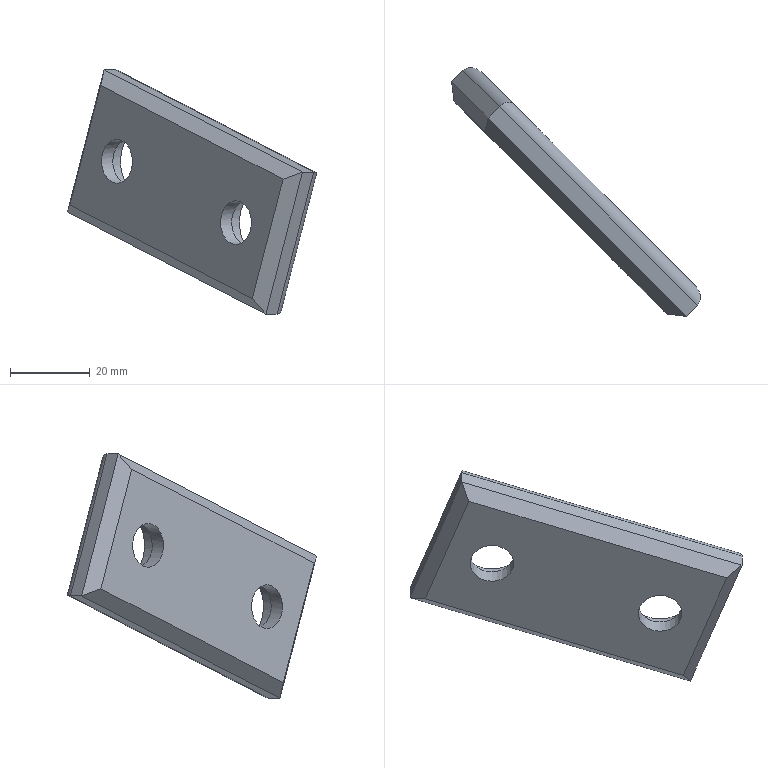Part | NX | features solid 2 | 1 solid | 20 faces | box 62.583 x 62.583 x 61.36 mm | volume 23446 mm3 | plane 12 | cylinder 8 | commonest cylinder face diameters 6 x4 11 x2 17.5 x2
STEP:
#1=CARTESIAN_POINT('',(-428.02,835.996,-99.293));
#2=VERTEX_POINT('',#1);
#3=CARTESIAN_POINT('',(-425.192,838.824,-99.293));
#4=VERTEX_POINT('',#3);
#5=CARTESIAN_POINT('',(-437.213,826.803,-99.293));
#6=DIRECTION('',(0.7071,0.7071,0.));
#7=VECTOR('',#6,1000.);
#8=LINE('',#5,#7);
#9=EDGE_CURVE('',#2,#4,#8,.T.);
#10=ORIENTED_EDGE('',*,*,#9,.F.);
#11=CARTESIAN_POINT('',(-418.83,826.806,-63.585));
#12=VERTEX_POINT('',#11);
#13=CARTESIAN_POINT('',(-428.02,835.996,-99.293));
#14=DIRECTION('',(0.2418,-0.2418,0.9397));
#15=VECTOR('',#14,1000.);
#16=LINE('',#13,#15);
#17=EDGE_CURVE('',#2,#12,#16,.T.);
#18=ORIENTED_EDGE('',*,*,#17,.T.);
#19=CARTESIAN_POINT('',(-416.002,829.634,-63.585));
#20=VERTEX_POINT('',#19);
#21=CARTESIAN_POINT('',(-428.022,817.613,-63.585));
#22=DIRECTION('',(0.7071,0.7071,0.));
#23=VECTOR('',#22,1000.);
#24=LINE('',#21,#23);
#25=EDGE_CURVE('',#12,#20,#24,.T.);
#26=ORIENTED_EDGE('',*,*,#25,.T.);
#27=CARTESIAN_POINT('',(-418.42,832.053,-72.982));
#28=DIRECTION('',(-0.2418,0.2418,-0.9397));
#29=VECTOR('',#28,1000.);
#30=LINE('',#27,#29);
#31=EDGE_CURVE('',#20,#4,#30,.T.);
#32=ORIENTED_EDGE('',*,*,#31,.T.);
#33=EDGE_LOOP('',(#10,#18,#26,#32));
#34=FACE_BOUND('',#33,.T.);
#35=CARTESIAN_POINT('',(-430.441,820.032,-72.982));
#36=DIRECTION('',(0.6645,-0.6645,-0.342));
#37=DIRECTION('',(0.7071,0.7071,0.));
#38=AXIS2_PLACEMENT_3D('',#35,#36,#37);
#39=PLANE('',#38);
#40=ADVANCED_FACE('',(#34),#39,.F.);
#41=CARTESIAN_POINT('',(-378.185,786.161,-124.945));
#42=VERTEX_POINT('',#41);
#43=CARTESIAN_POINT('',(-375.357,788.989,-124.945));
#44=VERTEX_POINT('',#43);
#45=CARTESIAN_POINT('',(-387.378,776.969,-124.945));
#46=DIRECTION('',(0.7071,0.7071,0.));
#47=VECTOR('',#46,1000.);
#48=LINE('',#45,#47);
#49=EDGE_CURVE('',#42,#44,#48,.T.);
#50=ORIENTED_EDGE('',*,*,#49,.F.);
#51=CARTESIAN_POINT('',(-428.02,835.996,-99.293));
#52=DIRECTION('',(-0.6645,0.6645,0.342));
#53=VECTOR('',#52,1000.);
#54=LINE('',#51,#53);
#55=EDGE_CURVE('',#42,#2,#54,.T.);
#56=ORIENTED_EDGE('',*,*,#55,.T.);
#57=ORIENTED_EDGE('',*,*,#9,.T.);
#58=CARTESIAN_POINT('',(-425.192,838.824,-99.293));
#59=DIRECTION('',(0.6645,-0.6645,-0.342));
#60=VECTOR('',#59,1000.);
#61=LINE('',#58,#60);
#62=EDGE_CURVE('',#4,#44,#61,.T.);
#63=ORIENTED_EDGE('',*,*,#62,.T.);
#64=EDGE_LOOP('',(#50,#56,#57,#63));
#65=FACE_BOUND('',#64,.T.);
#66=CARTESIAN_POINT('',(-437.213,826.803,-99.293));
#67=DIRECTION('',(0.2418,-0.2418,0.9397));
#68=DIRECTION('',(-0.7071,-0.7071,0.));
#69=AXIS2_PLACEMENT_3D('',#66,#67,#68);
#70=PLANE('',#69);
#71=ADVANCED_FACE('',(#65),#70,.F.);
#72=CARTESIAN_POINT('',(-368.995,776.971,-89.236));
#73=VERTEX_POINT('',#72);
#74=CARTESIAN_POINT('',(-366.167,779.799,-89.236));
#75=VERTEX_POINT('',#74);
#76=CARTESIAN_POINT('',(-378.188,767.779,-89.236));
#77=DIRECTION('',(0.7071,0.7071,0.));
#78=VECTOR('',#77,1000.);
#79=LINE('',#76,#78);
#80=EDGE_CURVE('',#73,#75,#79,.T.);
#81=ORIENTED_EDGE('',*,*,#80,.F.);
#82=CARTESIAN_POINT('',(-378.185,786.161,-124.945));
#83=DIRECTION('',(-0.2418,0.2418,-0.9397));
#84=VECTOR('',#83,1000.);
#85=LINE('',#82,#84);
#86=EDGE_CURVE('',#73,#42,#85,.T.);
#87=ORIENTED_EDGE('',*,*,#86,.T.);
#88=ORIENTED_EDGE('',*,*,#49,.T.);
#89=CARTESIAN_POINT('',(-375.357,788.989,-124.945));
#90=DIRECTION('',(0.2418,-0.2418,0.9397));
#91=VECTOR('',#90,1000.);
#92=LINE('',#89,#91);
#93=EDGE_CURVE('',#44,#75,#92,.T.);
#94=ORIENTED_EDGE('',*,*,#93,.T.);
#95=EDGE_LOOP('',(#81,#87,#88,#94));
#96=FACE_BOUND('',#95,.T.);
#97=CARTESIAN_POINT('',(-387.378,776.969,-124.945));
#98=DIRECTION('',(-0.6645,0.6645,0.342));
#99=DIRECTION('',(-0.7071,-0.7071,0.));
#100=AXIS2_PLACEMENT_3D('',#97,#98,#99);
#101=PLANE('',#100);
#102=ADVANCED_FACE('',(#96),#101,.F.);
#103=ORIENTED_EDGE('',*,*,#25,.F.);
#104=CARTESIAN_POINT('',(-418.83,826.806,-63.585));
#105=DIRECTION('',(0.6645,-0.6645,-0.342));
#106=VECTOR('',#105,1000.);
#107=LINE('',#104,#106);
#108=EDGE_CURVE('',#12,#73,#107,.T.);
#109=ORIENTED_EDGE('',*,*,#108,.T.);
#110=ORIENTED_EDGE('',*,*,#80,.T.);
#111=CARTESIAN_POINT('',(-366.167,779.799,-89.236));
#112=DIRECTION('',(-0.6645,0.6645,0.342));
#113=VECTOR('',#112,1000.);
#114=LINE('',#111,#113);
#115=EDGE_CURVE('',#75,#20,#114,.T.);
#116=ORIENTED_EDGE('',*,*,#115,.T.);
#117=EDGE_LOOP('',(#103,#109,#110,#116));
#118=FACE_BOUND('',#117,.T.);
#119=CARTESIAN_POINT('',(-378.188,767.779,-89.236));
#120=DIRECTION('',(-0.2418,0.2418,-0.9397));
#121=DIRECTION('',(0.6645,-0.6645,-0.342));
#122=AXIS2_PLACEMENT_3D('',#119,#120,#121);
#123=PLANE('',#122);
#124=ADVANCED_FACE('',(#118),#123,.F.);
#125=CARTESIAN_POINT('',(-427.423,831.155,-97.5));
#126=VERTEX_POINT('',#125);
#127=CARTESIAN_POINT('',(-381.575,785.308,-121.1));
#128=VERTEX_POINT('',#127);
#129=CARTESIAN_POINT('',(-379.581,783.314,-122.126));
#130=DIRECTION('',(0.6645,-0.6645,-0.342));
#131=VECTOR('',#130,1000.);
#132=LINE('',#129,#131);
#133=EDGE_CURVE('',#126,#128,#132,.T.);
#134=ORIENTED_EDGE('',*,*,#133,.T.);
#135=CARTESIAN_POINT('',(-373.836,777.569,-91.029));
#136=VERTEX_POINT('',#135);
#137=CARTESIAN_POINT('',(-375.529,779.261,-97.607));
#138=DIRECTION('',(0.2418,-0.2418,0.9397));
#139=VECTOR('',#138,1000.);
#140=LINE('',#137,#139);
#141=EDGE_CURVE('',#128,#136,#140,.T.);
#142=ORIENTED_EDGE('',*,*,#141,.T.);
#143=CARTESIAN_POINT('',(-419.684,823.416,-67.43));
#144=VERTEX_POINT('',#143);
#145=CARTESIAN_POINT('',(-421.677,825.41,-66.404));
#146=DIRECTION('',(-0.6645,0.6645,0.342));
#147=VECTOR('',#146,1000.);
#148=LINE('',#145,#147);
#149=EDGE_CURVE('',#136,#144,#148,.T.);
#150=ORIENTED_EDGE('',*,*,#149,.T.);
#151=CARTESIAN_POINT('',(-428.148,831.881,-100.319));
#152=DIRECTION('',(-0.2418,0.2418,-0.9397));
#153=VECTOR('',#152,1000.);
#154=LINE('',#151,#153);
#155=EDGE_CURVE('',#144,#126,#154,.T.);
#156=ORIENTED_EDGE('',*,*,#155,.T.);
#157=EDGE_LOOP('',(#134,#142,#150,#156));
#158=FACE_BOUND('',#157,.T.);
#159=CARTESIAN_POINT('',(-382.024,785.757,-103.841));
#160=VERTEX_POINT('',#159);
#161=CARTESIAN_POINT('',(-385.679,789.412,-101.96));
#162=DIRECTION('',(-0.7071,-0.7071,0.));
#163=DIRECTION('',(0.6645,-0.6645,-0.342));
#164=AXIS2_PLACEMENT_3D('',#161,#162,#163);
#165=CIRCLE('',#164,5.5);
#166=EDGE_CURVE('',#160,#160,#165,.T.);
#167=ORIENTED_EDGE('',*,*,#166,.F.);
#168=EDGE_LOOP('',(#167));
#169=FACE_BOUND('',#168,.T.);
#170=CARTESIAN_POINT('',(-411.925,815.658,-88.451));
#171=VERTEX_POINT('',#170);
#172=CARTESIAN_POINT('',(-415.58,819.312,-86.569));
#173=DIRECTION('',(-0.7071,-0.7071,0.));
#174=DIRECTION('',(0.6645,-0.6645,-0.342));
#175=AXIS2_PLACEMENT_3D('',#172,#173,#174);
#176=CIRCLE('',#175,5.5);
#177=EDGE_CURVE('',#171,#171,#176,.T.);
#178=ORIENTED_EDGE('',*,*,#177,.F.);
#179=EDGE_LOOP('',(#178));
#180=FACE_BOUND('',#179,.T.);
#181=CARTESIAN_POINT('',(-430.142,833.874,-99.293));
#182=DIRECTION('',(-0.7071,-0.7071,0.));
#183=DIRECTION('',(0.6645,-0.6645,-0.342));
#184=AXIS2_PLACEMENT_3D('',#181,#182,#183);
#185=PLANE('',#184);
#186=ADVANCED_FACE('',(#158,#169,#180),#185,.T.);
#187=CARTESIAN_POINT('',(-420.352,838.227,-97.5));
#188=VERTEX_POINT('',#187);
#189=CARTESIAN_POINT('',(-412.612,830.488,-67.43));
#190=VERTEX_POINT('',#189);
#191=CARTESIAN_POINT('',(-421.077,838.952,-100.319));
#192=DIRECTION('',(-0.2418,0.2418,-0.9397));
#193=VECTOR('',#192,1000.);
#194=LINE('',#191,#193);
#195=EDGE_CURVE('',#188,#190,#194,.F.);
#196=ORIENTED_EDGE('',*,*,#195,.T.);
#197=CARTESIAN_POINT('',(-366.765,784.64,-91.029));
#198=VERTEX_POINT('',#197);
#199=CARTESIAN_POINT('',(-414.606,832.481,-66.404));
#200=DIRECTION('',(-0.6645,0.6645,0.342));
#201=VECTOR('',#200,1000.);
#202=LINE('',#199,#201);
#203=EDGE_CURVE('',#190,#198,#202,.F.);
#204=ORIENTED_EDGE('',*,*,#203,.T.);
#205=CARTESIAN_POINT('',(-374.504,792.379,-121.1));
#206=VERTEX_POINT('',#205);
#207=CARTESIAN_POINT('',(-375.229,793.104,-123.919));
#208=DIRECTION('',(0.2418,-0.2418,0.9397));
#209=VECTOR('',#208,1000.);
#210=LINE('',#207,#209);
#211=EDGE_CURVE('',#198,#206,#210,.F.);
#212=ORIENTED_EDGE('',*,*,#211,.T.);
#213=CARTESIAN_POINT('',(-422.345,840.22,-96.474));
#214=DIRECTION('',(0.6645,-0.6645,-0.342));
#215=VECTOR('',#214,1000.);
#216=LINE('',#213,#215);
#217=EDGE_CURVE('',#206,#188,#216,.F.);
#218=ORIENTED_EDGE('',*,*,#217,.T.);
#219=EDGE_LOOP('',(#196,#204,#212,#218));
#220=FACE_BOUND('',#219,.T.);
#221=CARTESIAN_POINT('',(-372.794,790.669,-104.953));
#222=VERTEX_POINT('',#221);
#223=CARTESIAN_POINT('',(-378.608,796.483,-101.96));
#224=DIRECTION('',(-0.7071,-0.7071,0.));
#225=DIRECTION('',(0.6645,-0.6645,-0.342));
#226=AXIS2_PLACEMENT_3D('',#223,#224,#225);
#227=CIRCLE('',#226,8.75);
#228=EDGE_CURVE('',#222,#222,#227,.T.);
#229=ORIENTED_EDGE('',*,*,#228,.T.);
#230=EDGE_LOOP('',(#229));
#231=FACE_BOUND('',#230,.T.);
#232=CARTESIAN_POINT('',(-402.694,820.569,-89.562));
#233=VERTEX_POINT('',#232);
#234=CARTESIAN_POINT('',(-408.508,826.383,-86.569));
#235=DIRECTION('',(-0.7071,-0.7071,0.));
#236=DIRECTION('',(0.6645,-0.6645,-0.342));
#237=AXIS2_PLACEMENT_3D('',#234,#235,#236);
#238=CIRCLE('',#237,8.75);
#239=EDGE_CURVE('',#233,#233,#238,.T.);
#240=ORIENTED_EDGE('',*,*,#239,.T.);
#241=EDGE_LOOP('',(#240));
#242=FACE_BOUND('',#241,.T.);
#243=CARTESIAN_POINT('',(-423.07,840.945,-99.293));
#244=DIRECTION('',(-0.7071,-0.7071,0.));
#245=DIRECTION('',(0.6645,-0.6645,-0.342));
#246=AXIS2_PLACEMENT_3D('',#243,#244,#245);
#247=PLANE('',#246);
#248=ADVANCED_FACE('',(#220,#231,#242),#247,.F.);
#249=ORIENTED_EDGE('',*,*,#177,.T.);
#250=EDGE_LOOP('',(#249));
#251=FACE_BOUND('',#250,.T.);
#252=CARTESIAN_POINT('',(-408.862,818.252,-86.569));
#253=VERTEX_POINT('',#252);
#254=CARTESIAN_POINT('',(-412.751,822.141,-86.569));
#255=DIRECTION('',(-0.7071,-0.7071,0.));
#256=DIRECTION('',(0.7071,-0.7071,0.));
#257=AXIS2_PLACEMENT_3D('',#254,#255,#256);
#258=CIRCLE('',#257,5.5);
#259=EDGE_CURVE('',#253,#253,#258,.T.);
#260=ORIENTED_EDGE('',*,*,#259,.F.);
#261=EDGE_LOOP('',(#260));
#262=FACE_BOUND('',#261,.T.);
#263=CARTESIAN_POINT('',(-436.793,798.099,-86.569));
#264=DIRECTION('',(-0.7071,-0.7071,0.));
#265=DIRECTION('',(0.6645,-0.6645,-0.342));
#266=AXIS2_PLACEMENT_3D('',#263,#264,#265);
#267=CYLINDRICAL_SURFACE('',#266,5.5);
#268=ADVANCED_FACE('',(#251,#262),#267,.F.);
#269=ORIENTED_EDGE('',*,*,#259,.T.);
#270=EDGE_LOOP('',(#269));
#271=FACE_BOUND('',#270,.T.);
#272=CARTESIAN_POINT('',(-406.564,815.954,-86.569));
#273=VERTEX_POINT('',#272);
#274=CARTESIAN_POINT('',(-412.751,822.141,-86.569));
#275=DIRECTION('',(-0.7071,-0.7071,0.));
#276=DIRECTION('',(0.7071,-0.7071,0.));
#277=AXIS2_PLACEMENT_3D('',#274,#275,#276);
#278=CIRCLE('',#277,8.75);
#279=EDGE_CURVE('',#273,#273,#278,.T.);
#280=ORIENTED_EDGE('',*,*,#279,.F.);
#281=EDGE_LOOP('',(#280));
#282=FACE_BOUND('',#281,.T.);
#283=CARTESIAN_POINT('',(-412.751,822.141,-86.569));
#284=DIRECTION('',(-0.7071,-0.7071,0.));
#285=DIRECTION('',(0.6645,-0.6645,-0.342));
#286=AXIS2_PLACEMENT_3D('',#283,#284,#285);
#287=PLANE('',#286);
#288=ADVANCED_FACE('',(#271,#282),#287,.F.);
#289=ORIENTED_EDGE('',*,*,#279,.T.);
#290=EDGE_LOOP('',(#289));
#291=FACE_BOUND('',#290,.T.);
#292=ORIENTED_EDGE('',*,*,#239,.F.);
#293=EDGE_LOOP('',(#292));
#294=FACE_BOUND('',#293,.T.);
#295=CARTESIAN_POINT('',(-408.508,826.383,-86.569));
#296=DIRECTION('',(-0.7071,-0.7071,0.));
#297=DIRECTION('',(0.6645,-0.6645,-0.342));
#298=AXIS2_PLACEMENT_3D('',#295,#296,#297);
#299=CYLINDRICAL_SURFACE('',#298,8.75);
#300=ADVANCED_FACE('',(#291,#294),#299,.F.);
#301=ORIENTED_EDGE('',*,*,#166,.T.);
#302=EDGE_LOOP('',(#301));
#303=FACE_BOUND('',#302,.T.);
#304=CARTESIAN_POINT('',(-378.961,788.351,-101.96));
#305=VERTEX_POINT('',#304);
#306=CARTESIAN_POINT('',(-382.85,792.24,-101.96));
#307=DIRECTION('',(-0.7071,-0.7071,0.));
#308=DIRECTION('',(0.7071,-0.7071,0.));
#309=AXIS2_PLACEMENT_3D('',#306,#307,#308);
#310=CIRCLE('',#309,5.5);
#311=EDGE_CURVE('',#305,#305,#310,.T.);
#312=ORIENTED_EDGE('',*,*,#311,.F.);
#313=EDGE_LOOP('',(#312));
#314=FACE_BOUND('',#313,.T.);
#315=CARTESIAN_POINT('',(-406.892,768.198,-101.96));
#316=DIRECTION('',(-0.7071,-0.7071,0.));
#317=DIRECTION('',(0.6645,-0.6645,-0.342));
#318=AXIS2_PLACEMENT_3D('',#315,#316,#317);
#319=CYLINDRICAL_SURFACE('',#318,5.5);
#320=ADVANCED_FACE('',(#303,#314),#319,.F.);
#321=ORIENTED_EDGE('',*,*,#311,.T.);
#322=EDGE_LOOP('',(#321));
#323=FACE_BOUND('',#322,.T.);
#324=CARTESIAN_POINT('',(-376.663,786.053,-101.96));
#325=VERTEX_POINT('',#324);
#326=CARTESIAN_POINT('',(-382.85,792.24,-101.96));
#327=DIRECTION('',(-0.7071,-0.7071,0.));
#328=DIRECTION('',(0.7071,-0.7071,0.));
#329=AXIS2_PLACEMENT_3D('',#326,#327,#328);
#330=CIRCLE('',#329,8.75);
#331=EDGE_CURVE('',#325,#325,#330,.T.);
#332=ORIENTED_EDGE('',*,*,#331,.F.);
#333=EDGE_LOOP('',(#332));
#334=FACE_BOUND('',#333,.T.);
#335=CARTESIAN_POINT('',(-382.85,792.24,-101.96));
#336=DIRECTION('',(-0.7071,-0.7071,0.));
#337=DIRECTION('',(0.6645,-0.6645,-0.342));
#338=AXIS2_PLACEMENT_3D('',#335,#336,#337);
#339=PLANE('',#338);
#340=ADVANCED_FACE('',(#323,#334),#339,.F.);
#341=ORIENTED_EDGE('',*,*,#331,.T.);
#342=EDGE_LOOP('',(#341));
#343=FACE_BOUND('',#342,.T.);
#344=ORIENTED_EDGE('',*,*,#228,.F.);
#345=EDGE_LOOP('',(#344));
#346=FACE_BOUND('',#345,.T.);
#347=CARTESIAN_POINT('',(-378.608,796.483,-101.96));
#348=DIRECTION('',(-0.7071,-0.7071,0.));
#349=DIRECTION('',(0.6645,-0.6645,-0.342));
#350=AXIS2_PLACEMENT_3D('',#347,#348,#349);
#351=CYLINDRICAL_SURFACE('',#350,8.75);
#352=ADVANCED_FACE('',(#343,#346),#351,.F.);
#353=CARTESIAN_POINT('',(-422.473,836.105,-97.5));
#354=DIRECTION('',(0.2988,-0.2988,-0.9063));
#355=DIRECTION('',(-0.6409,0.6409,-0.4226));
#356=AXIS2_PLACEMENT_3D('',#353,#354,#355);
#357=ELLIPSE('',#356,4.243,3.);
#358=EDGE_CURVE('',#188,#4,#357,.F.);
#359=ORIENTED_EDGE('',*,*,#358,.F.);
#360=ORIENTED_EDGE('',*,*,#217,.F.);
#361=CARTESIAN_POINT('',(-376.625,790.257,-121.1));
#362=DIRECTION('',(0.6409,-0.6409,0.4226));
#363=DIRECTION('',(0.2988,-0.2988,-0.9063));
#364=AXIS2_PLACEMENT_3D('',#361,#362,#363);
#365=ELLIPSE('',#364,4.243,3.);
#366=EDGE_CURVE('',#44,#206,#365,.T.);
#367=ORIENTED_EDGE('',*,*,#366,.F.);
#368=ORIENTED_EDGE('',*,*,#62,.F.);
#369=EDGE_LOOP('',(#359,#360,#367,#368));
#370=FACE_BOUND('',#369,.T.);
#371=CARTESIAN_POINT('',(-424.466,838.099,-96.474));
#372=DIRECTION('',(0.6645,-0.6645,-0.342));
#373=DIRECTION('',(0.7071,0.7071,0.));
#374=AXIS2_PLACEMENT_3D('',#371,#372,#373);
#375=CYLINDRICAL_SURFACE('',#374,3.);
#376=ADVANCED_FACE('',(#370),#375,.T.);
#377=ORIENTED_EDGE('',*,*,#366,.T.);
#378=ORIENTED_EDGE('',*,*,#211,.F.);
#379=CARTESIAN_POINT('',(-368.886,782.518,-91.029));
#380=DIRECTION('',(-0.2988,0.2988,0.9063));
#381=DIRECTION('',(0.6409,-0.6409,0.4226));
#382=AXIS2_PLACEMENT_3D('',#379,#380,#381);
#383=ELLIPSE('',#382,4.243,3.);
#384=EDGE_CURVE('',#75,#198,#383,.T.);
#385=ORIENTED_EDGE('',*,*,#384,.F.);
#386=ORIENTED_EDGE('',*,*,#93,.F.);
#387=EDGE_LOOP('',(#377,#378,#385,#386));
#388=FACE_BOUND('',#387,.T.);
#389=CARTESIAN_POINT('',(-377.35,790.983,-123.919));
#390=DIRECTION('',(0.2418,-0.2418,0.9397));
#391=DIRECTION('',(-0.7071,-0.7071,0.));
#392=AXIS2_PLACEMENT_3D('',#389,#390,#391);
#393=CYLINDRICAL_SURFACE('',#392,3.);
#394=ADVANCED_FACE('',(#388),#393,.T.);
#395=ORIENTED_EDGE('',*,*,#358,.T.);
#396=ORIENTED_EDGE('',*,*,#31,.F.);
#397=CARTESIAN_POINT('',(-414.734,828.366,-67.43));
#398=DIRECTION('',(-0.6409,0.6409,-0.4226));
#399=DIRECTION('',(0.2988,-0.2988,-0.9063));
#400=AXIS2_PLACEMENT_3D('',#397,#398,#399);
#401=ELLIPSE('',#400,4.243,3.);
#402=EDGE_CURVE('',#190,#20,#401,.F.);
#403=ORIENTED_EDGE('',*,*,#402,.F.);
#404=ORIENTED_EDGE('',*,*,#195,.F.);
#405=EDGE_LOOP('',(#395,#396,#403,#404));
#406=FACE_BOUND('',#405,.T.);
#407=CARTESIAN_POINT('',(-416.427,830.059,-74.008));
#408=DIRECTION('',(-0.2418,0.2418,-0.9397));
#409=DIRECTION('',(0.7071,0.7071,0.));
#410=AXIS2_PLACEMENT_3D('',#407,#408,#409);
#411=CYLINDRICAL_SURFACE('',#410,3.);
#412=ADVANCED_FACE('',(#406),#411,.T.);
#413=ORIENTED_EDGE('',*,*,#384,.T.);
#414=ORIENTED_EDGE('',*,*,#203,.F.);
#415=ORIENTED_EDGE('',*,*,#402,.T.);
#416=ORIENTED_EDGE('',*,*,#115,.F.);
#417=EDGE_LOOP('',(#413,#414,#415,#416));
#418=FACE_BOUND('',#417,.T.);
#419=CARTESIAN_POINT('',(-366.892,780.525,-92.056));
#420=DIRECTION('',(-0.6645,0.6645,0.342));
#421=DIRECTION('',(-0.2418,0.2418,-0.9397));
#422=AXIS2_PLACEMENT_3D('',#419,#420,#421);
#423=CYLINDRICAL_SURFACE('',#422,3.);
#424=ADVANCED_FACE('',(#418),#423,.T.);
#425=CARTESIAN_POINT('',(-419.399,824.546,-66.148));
#426=DIRECTION('',(-0.1642,-0.6522,-0.74));
#427=VECTOR('',#426,1000.);
#428=LINE('',#425,#427);
#429=EDGE_CURVE('',#12,#144,#428,.T.);
#430=ORIENTED_EDGE('',*,*,#429,.F.);
#431=ORIENTED_EDGE('',*,*,#17,.F.);
#432=CARTESIAN_POINT('',(-427.622,832.769,-98.098));
#433=DIRECTION('',(0.115,-0.9315,0.3451));
#434=VECTOR('',#433,1000.);
#435=LINE('',#432,#434);
#436=EDGE_CURVE('',#126,#2,#435,.F.);
#437=ORIENTED_EDGE('',*,*,#436,.F.);
#438=ORIENTED_EDGE('',*,*,#155,.F.);
#439=EDGE_LOOP('',(#430,#431,#437,#438));
#440=FACE_BOUND('',#439,.T.);
#441=CARTESIAN_POINT('',(-428.148,831.881,-100.319));
#442=DIRECTION('',(-0.9698,-0.03015,0.2418));
#443=DIRECTION('',(-0.03015,-0.9698,-0.2418));
#444=AXIS2_PLACEMENT_3D('',#441,#442,#443);
#445=PLANE('',#444);
#446=ADVANCED_FACE('',(#440),#445,.T.);
#447=ORIENTED_EDGE('',*,*,#436,.T.);
#448=ORIENTED_EDGE('',*,*,#55,.F.);
#449=CARTESIAN_POINT('',(-408.688,778.48,-90.339));
#450=DIRECTION('',(-0.6522,-0.1642,0.74));
#451=VECTOR('',#450,1000.);
#452=LINE('',#449,#451);
#453=EDGE_CURVE('',#128,#42,#452,.F.);
#454=ORIENTED_EDGE('',*,*,#453,.F.);
#455=ORIENTED_EDGE('',*,*,#133,.F.);
#456=EDGE_LOOP('',(#447,#448,#454,#455));
#457=FACE_BOUND('',#456,.T.);
#458=CARTESIAN_POINT('',(-429.416,833.149,-96.474));
#459=DIRECTION('',(-0.671,-0.329,-0.6645));
#460=DIRECTION('',(0.329,0.671,-0.6645));
#461=AXIS2_PLACEMENT_3D('',#458,#459,#460);
#462=PLANE('',#461);
#463=ADVANCED_FACE('',(#457),#462,.T.);
#464=ORIENTED_EDGE('',*,*,#429,.T.);
#465=ORIENTED_EDGE('',*,*,#149,.F.);
#466=CARTESIAN_POINT('',(-412.558,782.349,-105.374));
#467=DIRECTION('',(0.9315,-0.115,0.3451));
#468=VECTOR('',#467,1000.);
#469=LINE('',#466,#468);
#470=EDGE_CURVE('',#73,#136,#469,.F.);
#471=ORIENTED_EDGE('',*,*,#470,.F.);
#472=ORIENTED_EDGE('',*,*,#108,.F.);
#473=EDGE_LOOP('',(#464,#465,#471,#472));
#474=FACE_BOUND('',#473,.T.);
#475=CARTESIAN_POINT('',(-421.677,825.41,-66.404));
#476=DIRECTION('',(-0.329,-0.671,0.6645));
#477=DIRECTION('',(-0.671,-0.329,-0.6645));
#478=AXIS2_PLACEMENT_3D('',#475,#476,#477);
#479=PLANE('',#478);
#480=ADVANCED_FACE('',(#474),#479,.T.);
#481=ORIENTED_EDGE('',*,*,#453,.T.);
#482=ORIENTED_EDGE('',*,*,#86,.F.);
#483=ORIENTED_EDGE('',*,*,#470,.T.);
#484=ORIENTED_EDGE('',*,*,#141,.F.);
#485=EDGE_LOOP('',(#481,#482,#483,#484));
#486=FACE_BOUND('',#485,.T.);
#487=CARTESIAN_POINT('',(-382.3,786.033,-123.919));
#488=DIRECTION('',(-0.03015,-0.9698,-0.2418));
#489=DIRECTION('',(0.9698,0.03015,-0.2418));
#490=AXIS2_PLACEMENT_3D('',#487,#488,#489);
#491=PLANE('',#490);
#492=ADVANCED_FACE('',(#486),#491,.T.);
#493=CLOSED_SHELL('',(#40,#71,#102,#124,#186,#248,#268,#288,#300,#320,#340,#352,#376,#394,#412,#424,#446,#463,#480,#492));
#494=MANIFOLD_SOLID_BREP('',#493);
#495=(LENGTH_UNIT()NAMED_UNIT(*)SI_UNIT(.MILLI.,.METRE.));
#496=UNCERTAINTY_MEASURE_WITH_UNIT(LENGTH_MEASURE(0.00001),#495,'','');
#497=(NAMED_UNIT(*)PLANE_ANGLE_UNIT()SI_UNIT($,.RADIAN.));
#498=(NAMED_UNIT(*)SI_UNIT($,.STERADIAN.)SOLID_ANGLE_UNIT());
#499=(GEOMETRIC_REPRESENTATION_CONTEXT(3)GLOBAL_UNCERTAINTY_ASSIGNED_CONTEXT((#496))GLOBAL_UNIT_ASSIGNED_CONTEXT((#495,#497,#498))REPRESENTATION_CONTEXT('',''));
#500=ADVANCED_BREP_SHAPE_REPRESENTATION('',(#494),#499);